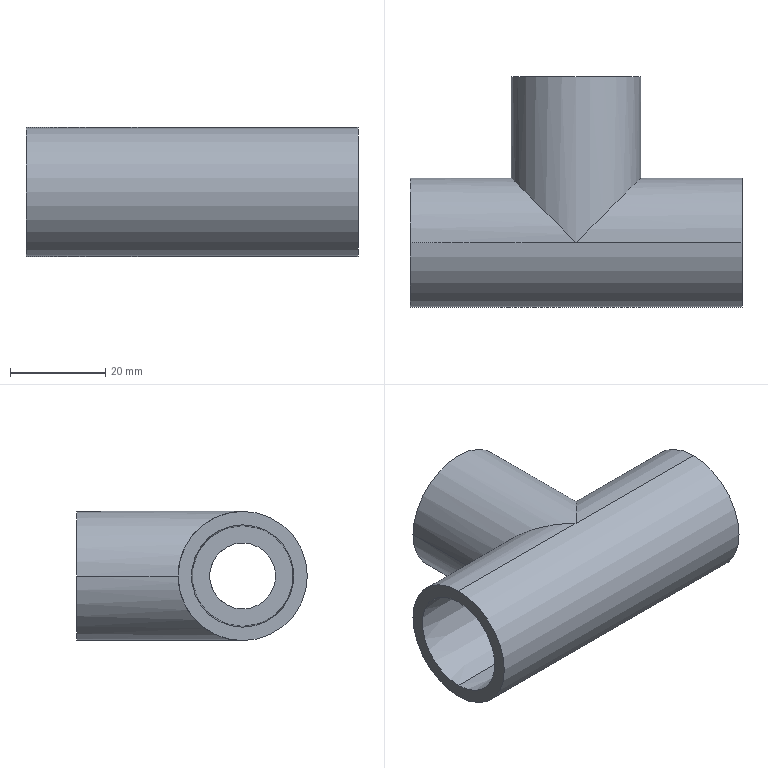Part | SolidWorks | features BaseBody 1 | 1 solid | 49 faces | box 69.85 x 48.514 x 27.178 mm | volume 26765 mm3 | cone 31 | cylinder 9 | plane 6 | spline 3 | commonest cylinder face diameters 27.178 x5 12.484 x2 13.868 x2